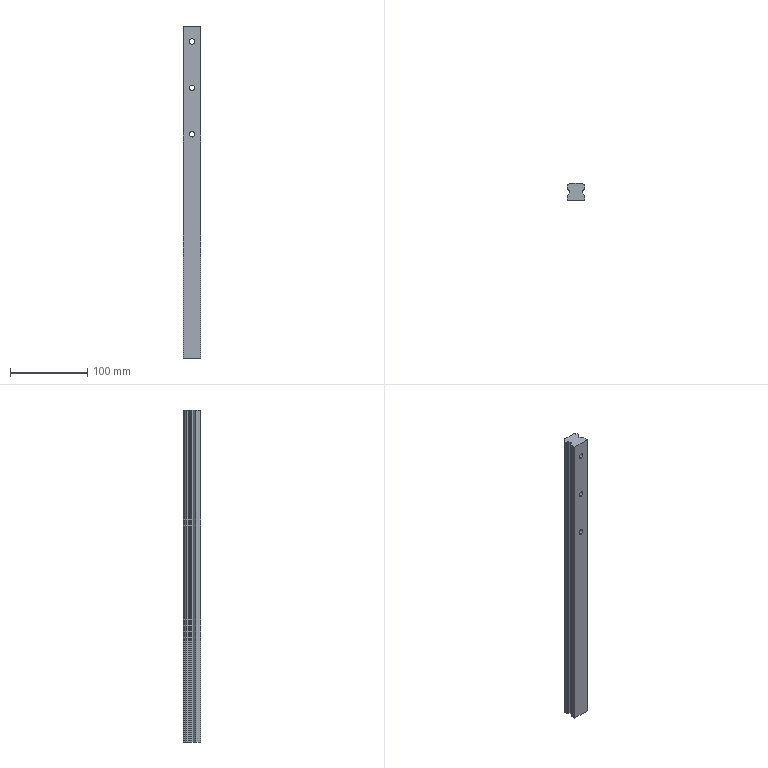Part | STEP file | 1 solid | 41 faces | box 23 x 22 x 429 mm | volume 189571 mm3 | plane 23 | cylinder 18 | commonest cylinder face diameters 2.258 x6 7 x6 11 x6
STEP:
#1=CARTESIAN_POINT('',(0.,-5.6,56.5));
#2=VERTEX_POINT('',#1);
#3=CARTESIAN_POINT('',(0.,-5.6,63.5));
#4=VERTEX_POINT('',#3);
#5=CARTESIAN_POINT('',(0.,-5.6,60.));
#6=DIRECTION('',(0.,1.,0.));
#7=DIRECTION('',(0.,0.,1.));
#8=AXIS2_PLACEMENT_3D('',#5,#6,#7);
#9=CIRCLE('',#8,3.5);
#10=EDGE_CURVE('',#2,#4,#9,.T.);
#11=ORIENTED_EDGE('',*,*,#10,.F.);
#12=CARTESIAN_POINT('',(0.,7.4,56.5));
#13=VERTEX_POINT('',#12);
#14=CARTESIAN_POINT('',(0.,16.4,56.5));
#15=DIRECTION('',(0.,1.,0.));
#16=VECTOR('',#15,1000.);
#17=LINE('',#14,#16);
#18=EDGE_CURVE('',#2,#13,#17,.T.);
#19=ORIENTED_EDGE('',*,*,#18,.T.);
#20=CARTESIAN_POINT('',(0.,7.4,63.5));
#21=VERTEX_POINT('',#20);
#22=CARTESIAN_POINT('',(0.,7.4,60.));
#23=DIRECTION('',(0.,-1.,0.));
#24=DIRECTION('',(0.,0.,1.));
#25=AXIS2_PLACEMENT_3D('',#22,#23,#24);
#26=CIRCLE('',#25,3.5);
#27=EDGE_CURVE('',#21,#13,#26,.T.);
#28=ORIENTED_EDGE('',*,*,#27,.F.);
#29=CARTESIAN_POINT('',(0.,16.4,63.5));
#30=DIRECTION('',(0.,1.,0.));
#31=VECTOR('',#30,1000.);
#32=LINE('',#29,#31);
#33=EDGE_CURVE('',#4,#21,#32,.T.);
#34=ORIENTED_EDGE('',*,*,#33,.F.);
#35=EDGE_LOOP('',(#11,#19,#28,#34));
#36=FACE_OUTER_BOUND('',#35,.T.);
#37=CARTESIAN_POINT('',(0.,16.4,60.));
#38=DIRECTION('',(0.,1.,0.));
#39=DIRECTION('',(0.,0.,1.));
#40=AXIS2_PLACEMENT_3D('',#37,#38,#39);
#41=CYLINDRICAL_SURFACE('',#40,3.5);
#42=ADVANCED_FACE('',(#36),#41,.F.);
#43=CARTESIAN_POINT('',(0.,-5.6,-3.5));
#44=VERTEX_POINT('',#43);
#45=CARTESIAN_POINT('',(0.,-5.6,3.5));
#46=VERTEX_POINT('',#45);
#47=CARTESIAN_POINT('',(0.,-5.6,0.));
#48=DIRECTION('',(0.,1.,0.));
#49=DIRECTION('',(0.,0.,1.));
#50=AXIS2_PLACEMENT_3D('',#47,#48,#49);
#51=CIRCLE('',#50,3.5);
#52=EDGE_CURVE('',#44,#46,#51,.T.);
#53=ORIENTED_EDGE('',*,*,#52,.F.);
#54=CARTESIAN_POINT('',(0.,7.4,-3.5));
#55=VERTEX_POINT('',#54);
#56=CARTESIAN_POINT('',(0.,16.4,-3.5));
#57=DIRECTION('',(0.,1.,0.));
#58=VECTOR('',#57,1000.);
#59=LINE('',#56,#58);
#60=EDGE_CURVE('',#44,#55,#59,.T.);
#61=ORIENTED_EDGE('',*,*,#60,.T.);
#62=CARTESIAN_POINT('',(0.,7.4,3.5));
#63=VERTEX_POINT('',#62);
#64=CARTESIAN_POINT('',(0.,7.4,0.));
#65=DIRECTION('',(0.,-1.,0.));
#66=DIRECTION('',(0.,0.,1.));
#67=AXIS2_PLACEMENT_3D('',#64,#65,#66);
#68=CIRCLE('',#67,3.5);
#69=EDGE_CURVE('',#63,#55,#68,.T.);
#70=ORIENTED_EDGE('',*,*,#69,.F.);
#71=CARTESIAN_POINT('',(0.,16.4,3.5));
#72=DIRECTION('',(0.,1.,0.));
#73=VECTOR('',#72,1000.);
#74=LINE('',#71,#73);
#75=EDGE_CURVE('',#46,#63,#74,.T.);
#76=ORIENTED_EDGE('',*,*,#75,.F.);
#77=EDGE_LOOP('',(#53,#61,#70,#76));
#78=FACE_OUTER_BOUND('',#77,.T.);
#79=CARTESIAN_POINT('',(0.,16.4,0.));
#80=DIRECTION('',(0.,1.,0.));
#81=DIRECTION('',(0.,0.,1.));
#82=AXIS2_PLACEMENT_3D('',#79,#80,#81);
#83=CYLINDRICAL_SURFACE('',#82,3.5);
#84=ADVANCED_FACE('',(#78),#83,.F.);
#85=CARTESIAN_POINT('',(0.,-5.6,-63.5));
#86=VERTEX_POINT('',#85);
#87=CARTESIAN_POINT('',(0.,-5.6,-56.5));
#88=VERTEX_POINT('',#87);
#89=CARTESIAN_POINT('',(0.,-5.6,-60.));
#90=DIRECTION('',(0.,1.,0.));
#91=DIRECTION('',(0.,0.,1.));
#92=AXIS2_PLACEMENT_3D('',#89,#90,#91);
#93=CIRCLE('',#92,3.5);
#94=EDGE_CURVE('',#86,#88,#93,.T.);
#95=ORIENTED_EDGE('',*,*,#94,.F.);
#96=CARTESIAN_POINT('',(0.,7.4,-63.5));
#97=VERTEX_POINT('',#96);
#98=CARTESIAN_POINT('',(0.,16.4,-63.5));
#99=DIRECTION('',(0.,1.,0.));
#100=VECTOR('',#99,1000.);
#101=LINE('',#98,#100);
#102=EDGE_CURVE('',#86,#97,#101,.T.);
#103=ORIENTED_EDGE('',*,*,#102,.T.);
#104=CARTESIAN_POINT('',(0.,7.4,-56.5));
#105=VERTEX_POINT('',#104);
#106=CARTESIAN_POINT('',(0.,7.4,-60.));
#107=DIRECTION('',(0.,-1.,0.));
#108=DIRECTION('',(0.,0.,1.));
#109=AXIS2_PLACEMENT_3D('',#106,#107,#108);
#110=CIRCLE('',#109,3.5);
#111=EDGE_CURVE('',#105,#97,#110,.T.);
#112=ORIENTED_EDGE('',*,*,#111,.F.);
#113=CARTESIAN_POINT('',(0.,16.4,-56.5));
#114=DIRECTION('',(0.,1.,0.));
#115=VECTOR('',#114,1000.);
#116=LINE('',#113,#115);
#117=EDGE_CURVE('',#88,#105,#116,.T.);
#118=ORIENTED_EDGE('',*,*,#117,.F.);
#119=EDGE_LOOP('',(#95,#103,#112,#118));
#120=FACE_OUTER_BOUND('',#119,.T.);
#121=CARTESIAN_POINT('',(0.,16.4,-60.));
#122=DIRECTION('',(0.,1.,0.));
#123=DIRECTION('',(0.,0.,1.));
#124=AXIS2_PLACEMENT_3D('',#121,#122,#123);
#125=CYLINDRICAL_SURFACE('',#124,3.5);
#126=ADVANCED_FACE('',(#120),#125,.F.);
#127=CARTESIAN_POINT('',(-9.204,7.727,-349.));
#128=VERTEX_POINT('',#127);
#129=CARTESIAN_POINT('',(-10.352,8.856,-349.));
#130=VERTEX_POINT('',#129);
#131=CARTESIAN_POINT('',(-10.333,7.727,-349.));
#132=DIRECTION('',(0.,0.,1.));
#133=DIRECTION('',(-1.,0.,0.));
#134=AXIS2_PLACEMENT_3D('',#131,#132,#133);
#135=CIRCLE('',#134,1.129);
#136=EDGE_CURVE('',#128,#130,#135,.T.);
#137=ORIENTED_EDGE('',*,*,#136,.F.);
#138=CARTESIAN_POINT('',(-9.204,7.727,80.));
#139=VERTEX_POINT('',#138);
#140=CARTESIAN_POINT('',(-9.204,7.727,-80.));
#141=DIRECTION('',(0.,0.,1.));
#142=VECTOR('',#141,1000.);
#143=LINE('',#140,#142);
#144=EDGE_CURVE('',#128,#139,#143,.T.);
#145=ORIENTED_EDGE('',*,*,#144,.T.);
#146=CARTESIAN_POINT('',(-10.352,8.856,80.));
#147=VERTEX_POINT('',#146);
#148=CARTESIAN_POINT('',(-10.333,7.727,80.));
#149=DIRECTION('',(0.,0.,-1.));
#150=DIRECTION('',(1.,0.,0.));
#151=AXIS2_PLACEMENT_3D('',#148,#149,#150);
#152=CIRCLE('',#151,1.129);
#153=EDGE_CURVE('',#147,#139,#152,.T.);
#154=ORIENTED_EDGE('',*,*,#153,.F.);
#155=CARTESIAN_POINT('',(-10.352,8.856,-80.));
#156=DIRECTION('',(0.,0.,1.));
#157=VECTOR('',#156,1000.);
#158=LINE('',#155,#157);
#159=EDGE_CURVE('',#130,#147,#158,.T.);
#160=ORIENTED_EDGE('',*,*,#159,.F.);
#161=EDGE_LOOP('',(#137,#145,#154,#160));
#162=FACE_OUTER_BOUND('',#161,.T.);
#163=CARTESIAN_POINT('',(-10.333,7.727,-80.));
#164=DIRECTION('',(0.,0.,1.));
#165=DIRECTION('',(1.,0.,0.));
#166=AXIS2_PLACEMENT_3D('',#163,#164,#165);
#167=CYLINDRICAL_SURFACE('',#166,1.129);
#168=ADVANCED_FACE('',(#162),#167,.F.);
#169=CARTESIAN_POINT('',(-9.204,15.233,-349.));
#170=VERTEX_POINT('',#169);
#171=CARTESIAN_POINT('',(-9.204,15.252,-349.));
#172=VERTEX_POINT('',#171);
#173=CARTESIAN_POINT('',(-10.333,15.233,-349.));
#174=DIRECTION('',(0.,0.,1.));
#175=DIRECTION('',(-1.,0.,0.));
#176=AXIS2_PLACEMENT_3D('',#173,#174,#175);
#177=CIRCLE('',#176,1.129);
#178=EDGE_CURVE('',#170,#172,#177,.T.);
#179=ORIENTED_EDGE('',*,*,#178,.F.);
#180=CARTESIAN_POINT('',(-9.204,15.233,80.));
#181=VERTEX_POINT('',#180);
#182=CARTESIAN_POINT('',(-9.204,15.233,-80.));
#183=DIRECTION('',(0.,0.,1.));
#184=VECTOR('',#183,1000.);
#185=LINE('',#182,#184);
#186=EDGE_CURVE('',#170,#181,#185,.T.);
#187=ORIENTED_EDGE('',*,*,#186,.T.);
#188=CARTESIAN_POINT('',(-9.204,15.252,80.));
#189=VERTEX_POINT('',#188);
#190=CARTESIAN_POINT('',(-10.333,15.233,80.));
#191=DIRECTION('',(0.,0.,-1.));
#192=DIRECTION('',(1.,0.,0.));
#193=AXIS2_PLACEMENT_3D('',#190,#191,#192);
#194=CIRCLE('',#193,1.129);
#195=EDGE_CURVE('',#189,#181,#194,.T.);
#196=ORIENTED_EDGE('',*,*,#195,.F.);
#197=CARTESIAN_POINT('',(-9.204,15.252,-80.));
#198=DIRECTION('',(0.,0.,1.));
#199=VECTOR('',#198,1000.);
#200=LINE('',#197,#199);
#201=EDGE_CURVE('',#172,#189,#200,.T.);
#202=ORIENTED_EDGE('',*,*,#201,.F.);
#203=EDGE_LOOP('',(#179,#187,#196,#202));
#204=FACE_OUTER_BOUND('',#203,.T.);
#205=CARTESIAN_POINT('',(-10.333,15.233,-80.));
#206=DIRECTION('',(0.,0.,1.));
#207=DIRECTION('',(1.,0.,0.));
#208=AXIS2_PLACEMENT_3D('',#205,#206,#207);
#209=CYLINDRICAL_SURFACE('',#208,1.129);
#210=ADVANCED_FACE('',(#204),#209,.F.);
#211=CARTESIAN_POINT('',(0.,7.4,65.5));
#212=VERTEX_POINT('',#211);
#213=CARTESIAN_POINT('',(0.,7.4,54.5));
#214=VERTEX_POINT('',#213);
#215=CARTESIAN_POINT('',(0.,7.4,60.));
#216=DIRECTION('',(0.,-1.,0.));
#217=DIRECTION('',(0.,0.,1.));
#218=AXIS2_PLACEMENT_3D('',#215,#216,#217);
#219=CIRCLE('',#218,5.5);
#220=EDGE_CURVE('',#212,#214,#219,.T.);
#221=ORIENTED_EDGE('',*,*,#220,.T.);
#222=CARTESIAN_POINT('',(0.,16.4,54.5));
#223=VERTEX_POINT('',#222);
#224=CARTESIAN_POINT('',(0.,16.4,54.5));
#225=DIRECTION('',(0.,1.,0.));
#226=VECTOR('',#225,1000.);
#227=LINE('',#224,#226);
#228=EDGE_CURVE('',#214,#223,#227,.T.);
#229=ORIENTED_EDGE('',*,*,#228,.T.);
#230=CARTESIAN_POINT('',(0.,16.4,65.5));
#231=VERTEX_POINT('',#230);
#232=CARTESIAN_POINT('',(0.,16.4,60.));
#233=DIRECTION('',(0.,-1.,0.));
#234=DIRECTION('',(0.,0.,1.));
#235=AXIS2_PLACEMENT_3D('',#232,#233,#234);
#236=CIRCLE('',#235,5.5);
#237=EDGE_CURVE('',#231,#223,#236,.T.);
#238=ORIENTED_EDGE('',*,*,#237,.F.);
#239=CARTESIAN_POINT('',(0.,16.4,65.5));
#240=DIRECTION('',(0.,1.,0.));
#241=VECTOR('',#240,1000.);
#242=LINE('',#239,#241);
#243=EDGE_CURVE('',#212,#231,#242,.T.);
#244=ORIENTED_EDGE('',*,*,#243,.F.);
#245=EDGE_LOOP('',(#221,#229,#238,#244));
#246=FACE_OUTER_BOUND('',#245,.T.);
#247=CARTESIAN_POINT('',(0.,16.4,60.));
#248=DIRECTION('',(0.,1.,0.));
#249=DIRECTION('',(0.,0.,1.));
#250=AXIS2_PLACEMENT_3D('',#247,#248,#249);
#251=CYLINDRICAL_SURFACE('',#250,5.5);
#252=ADVANCED_FACE('',(#246),#251,.F.);
#253=CARTESIAN_POINT('',(0.,7.4,5.5));
#254=VERTEX_POINT('',#253);
#255=CARTESIAN_POINT('',(0.,7.4,-5.5));
#256=VERTEX_POINT('',#255);
#257=CARTESIAN_POINT('',(0.,7.4,0.));
#258=DIRECTION('',(0.,-1.,0.));
#259=DIRECTION('',(0.,0.,1.));
#260=AXIS2_PLACEMENT_3D('',#257,#258,#259);
#261=CIRCLE('',#260,5.5);
#262=EDGE_CURVE('',#254,#256,#261,.T.);
#263=ORIENTED_EDGE('',*,*,#262,.T.);
#264=CARTESIAN_POINT('',(0.,16.4,-5.5));
#265=VERTEX_POINT('',#264);
#266=CARTESIAN_POINT('',(0.,16.4,-5.5));
#267=DIRECTION('',(0.,1.,0.));
#268=VECTOR('',#267,1000.);
#269=LINE('',#266,#268);
#270=EDGE_CURVE('',#256,#265,#269,.T.);
#271=ORIENTED_EDGE('',*,*,#270,.T.);
#272=CARTESIAN_POINT('',(0.,16.4,5.5));
#273=VERTEX_POINT('',#272);
#274=CARTESIAN_POINT('',(0.,16.4,0.));
#275=DIRECTION('',(0.,-1.,0.));
#276=DIRECTION('',(0.,0.,1.));
#277=AXIS2_PLACEMENT_3D('',#274,#275,#276);
#278=CIRCLE('',#277,5.5);
#279=EDGE_CURVE('',#273,#265,#278,.T.);
#280=ORIENTED_EDGE('',*,*,#279,.F.);
#281=CARTESIAN_POINT('',(0.,16.4,5.5));
#282=DIRECTION('',(0.,1.,0.));
#283=VECTOR('',#282,1000.);
#284=LINE('',#281,#283);
#285=EDGE_CURVE('',#254,#273,#284,.T.);
#286=ORIENTED_EDGE('',*,*,#285,.F.);
#287=EDGE_LOOP('',(#263,#271,#280,#286));
#288=FACE_OUTER_BOUND('',#287,.T.);
#289=CARTESIAN_POINT('',(0.,16.4,0.));
#290=DIRECTION('',(0.,1.,0.));
#291=DIRECTION('',(0.,0.,1.));
#292=AXIS2_PLACEMENT_3D('',#289,#290,#291);
#293=CYLINDRICAL_SURFACE('',#292,5.5);
#294=ADVANCED_FACE('',(#288),#293,.F.);
#295=CARTESIAN_POINT('',(0.,7.4,-54.5));
#296=VERTEX_POINT('',#295);
#297=CARTESIAN_POINT('',(0.,7.4,-65.5));
#298=VERTEX_POINT('',#297);
#299=CARTESIAN_POINT('',(0.,7.4,-60.));
#300=DIRECTION('',(0.,-1.,0.));
#301=DIRECTION('',(0.,0.,1.));
#302=AXIS2_PLACEMENT_3D('',#299,#300,#301);
#303=CIRCLE('',#302,5.5);
#304=EDGE_CURVE('',#296,#298,#303,.T.);
#305=ORIENTED_EDGE('',*,*,#304,.T.);
#306=CARTESIAN_POINT('',(0.,16.4,-65.5));
#307=VERTEX_POINT('',#306);
#308=CARTESIAN_POINT('',(0.,16.4,-65.5));
#309=DIRECTION('',(0.,1.,0.));
#310=VECTOR('',#309,1000.);
#311=LINE('',#308,#310);
#312=EDGE_CURVE('',#298,#307,#311,.T.);
#313=ORIENTED_EDGE('',*,*,#312,.T.);
#314=CARTESIAN_POINT('',(0.,16.4,-54.5));
#315=VERTEX_POINT('',#314);
#316=CARTESIAN_POINT('',(0.,16.4,-60.));
#317=DIRECTION('',(0.,-1.,0.));
#318=DIRECTION('',(0.,0.,1.));
#319=AXIS2_PLACEMENT_3D('',#316,#317,#318);
#320=CIRCLE('',#319,5.5);
#321=EDGE_CURVE('',#315,#307,#320,.T.);
#322=ORIENTED_EDGE('',*,*,#321,.F.);
#323=CARTESIAN_POINT('',(0.,16.4,-54.5));
#324=DIRECTION('',(0.,1.,0.));
#325=VECTOR('',#324,1000.);
#326=LINE('',#323,#325);
#327=EDGE_CURVE('',#296,#315,#326,.T.);
#328=ORIENTED_EDGE('',*,*,#327,.F.);
#329=EDGE_LOOP('',(#305,#313,#322,#328));
#330=FACE_OUTER_BOUND('',#329,.T.);
#331=CARTESIAN_POINT('',(0.,16.4,-60.));
#332=DIRECTION('',(0.,1.,0.));
#333=DIRECTION('',(0.,0.,1.));
#334=AXIS2_PLACEMENT_3D('',#331,#332,#333);
#335=CYLINDRICAL_SURFACE('',#334,5.5);
#336=ADVANCED_FACE('',(#330),#335,.F.);
#337=CARTESIAN_POINT('',(-11.5,-5.6,80.));
#338=VERTEX_POINT('',#337);
#339=CARTESIAN_POINT('',(-11.5,-5.6,-349.));
#340=VERTEX_POINT('',#339);
#341=CARTESIAN_POINT('',(-11.5,-5.6,-80.));
#342=DIRECTION('',(0.,0.,-1.));
#343=VECTOR('',#342,1000.);
#344=LINE('',#341,#343);
#345=EDGE_CURVE('',#338,#340,#344,.T.);
#346=ORIENTED_EDGE('',*,*,#345,.T.);
#347=CARTESIAN_POINT('',(11.5,-5.6,-349.));
#348=VERTEX_POINT('',#347);
#349=CARTESIAN_POINT('',(11.5,-5.6,-349.));
#350=DIRECTION('',(-1.,0.,0.));
#351=VECTOR('',#350,1000.);
#352=LINE('',#349,#351);
#353=EDGE_CURVE('',#348,#340,#352,.T.);
#354=ORIENTED_EDGE('',*,*,#353,.F.);
#355=CARTESIAN_POINT('',(11.5,-5.6,80.));
#356=VERTEX_POINT('',#355);
#357=CARTESIAN_POINT('',(11.5,-5.6,-80.));
#358=DIRECTION('',(0.,0.,1.));
#359=VECTOR('',#358,1000.);
#360=LINE('',#357,#359);
#361=EDGE_CURVE('',#348,#356,#360,.T.);
#362=ORIENTED_EDGE('',*,*,#361,.T.);
#363=CARTESIAN_POINT('',(-11.5,-5.6,80.));
#364=DIRECTION('',(-1.,0.,0.));
#365=VECTOR('',#364,1000.);
#366=LINE('',#363,#365);
#367=EDGE_CURVE('',#356,#338,#366,.T.);
#368=ORIENTED_EDGE('',*,*,#367,.T.);
#369=EDGE_LOOP('',(#346,#354,#362,#368));
#370=FACE_OUTER_BOUND('',#369,.T.);
#371=CARTESIAN_POINT('',(0.,-5.6,60.));
#372=DIRECTION('',(0.,1.,0.));
#373=DIRECTION('',(0.,0.,1.));
#374=AXIS2_PLACEMENT_3D('',#371,#372,#373);
#375=CIRCLE('',#374,3.5);
#376=EDGE_CURVE('',#4,#2,#375,.T.);
#377=ORIENTED_EDGE('',*,*,#376,.T.);
#378=ORIENTED_EDGE('',*,*,#10,.T.);
#379=EDGE_LOOP('',(#377,#378));
#380=FACE_BOUND('',#379,.T.);
#381=CARTESIAN_POINT('',(0.,-5.6,0.));
#382=DIRECTION('',(0.,1.,0.));
#383=DIRECTION('',(0.,0.,1.));
#384=AXIS2_PLACEMENT_3D('',#381,#382,#383);
#385=CIRCLE('',#384,3.5);
#386=EDGE_CURVE('',#46,#44,#385,.T.);
#387=ORIENTED_EDGE('',*,*,#386,.T.);
#388=ORIENTED_EDGE('',*,*,#52,.T.);
#389=EDGE_LOOP('',(#387,#388));
#390=FACE_BOUND('',#389,.T.);
#391=CARTESIAN_POINT('',(0.,-5.6,-60.));
#392=DIRECTION('',(0.,1.,0.));
#393=DIRECTION('',(0.,0.,1.));
#394=AXIS2_PLACEMENT_3D('',#391,#392,#393);
#395=CIRCLE('',#394,3.5);
#396=EDGE_CURVE('',#88,#86,#395,.T.);
#397=ORIENTED_EDGE('',*,*,#396,.T.);
#398=ORIENTED_EDGE('',*,*,#94,.T.);
#399=EDGE_LOOP('',(#397,#398));
#400=FACE_BOUND('',#399,.T.);
#401=CARTESIAN_POINT('',(-11.5,-5.6,-80.));
#402=DIRECTION('',(0.,-1.,0.));
#403=DIRECTION('',(0.,0.,-1.));
#404=AXIS2_PLACEMENT_3D('',#401,#402,#403);
#405=PLANE('',#404);
#406=ADVANCED_FACE('',(#370,#380,#390,#400),#405,.T.);
#407=CARTESIAN_POINT('',(-11.5,0.575,80.));
#408=VERTEX_POINT('',#407);
#409=CARTESIAN_POINT('',(-11.5,0.575,-349.));
#410=VERTEX_POINT('',#409);
#411=CARTESIAN_POINT('',(-11.5,0.575,-80.));
#412=DIRECTION('',(0.,0.,-1.));
#413=VECTOR('',#412,1000.);
#414=LINE('',#411,#413);
#415=EDGE_CURVE('',#408,#410,#414,.T.);
#416=ORIENTED_EDGE('',*,*,#415,.T.);
#417=CARTESIAN_POINT('',(-11.5,-5.6,-349.));
#418=DIRECTION('',(0.,1.,0.));
#419=VECTOR('',#418,1000.);
#420=LINE('',#417,#419);
#421=EDGE_CURVE('',#340,#410,#420,.T.);
#422=ORIENTED_EDGE('',*,*,#421,.F.);
#423=ORIENTED_EDGE('',*,*,#345,.F.);
#424=CARTESIAN_POINT('',(-11.5,-5.6,80.));
#425=DIRECTION('',(0.,1.,0.));
#426=VECTOR('',#425,1000.);
#427=LINE('',#424,#426);
#428=EDGE_CURVE('',#338,#408,#427,.T.);
#429=ORIENTED_EDGE('',*,*,#428,.T.);
#430=EDGE_LOOP('',(#416,#422,#423,#429));
#431=FACE_OUTER_BOUND('',#430,.T.);
#432=CARTESIAN_POINT('',(-11.5,-5.6,-80.));
#433=DIRECTION('',(-1.,0.,0.));
#434=DIRECTION('',(0.,-1.,0.));
#435=AXIS2_PLACEMENT_3D('',#432,#433,#434);
#436=PLANE('',#435);
#437=ADVANCED_FACE('',(#431),#436,.T.);
#438=CARTESIAN_POINT('',(10.352,14.104,80.));
#439=VERTEX_POINT('',#438);
#440=CARTESIAN_POINT('',(11.5,12.956,80.));
#441=VERTEX_POINT('',#440);
#442=CARTESIAN_POINT('',(11.5,12.956,80.));
#443=DIRECTION('',(0.7071,-0.7071,0.));
#444=VECTOR('',#443,1000.);
#445=LINE('',#442,#444);
#446=EDGE_CURVE('',#439,#441,#445,.T.);
#447=ORIENTED_EDGE('',*,*,#446,.F.);
#448=CARTESIAN_POINT('',(9.204,15.252,80.));
#449=VERTEX_POINT('',#448);
#450=CARTESIAN_POINT('',(10.333,15.233,80.));
#451=DIRECTION('',(0.,0.,-1.));
#452=DIRECTION('',(1.,0.,0.));
#453=AXIS2_PLACEMENT_3D('',#450,#451,#452);
#454=CIRCLE('',#453,1.129);
#455=EDGE_CURVE('',#439,#449,#454,.T.);
#456=ORIENTED_EDGE('',*,*,#455,.T.);
#457=CARTESIAN_POINT('',(8.056,16.4,80.));
#458=VERTEX_POINT('',#457);
#459=CARTESIAN_POINT('',(9.204,15.252,80.));
#460=DIRECTION('',(0.7071,-0.7071,0.));
#461=VECTOR('',#460,1000.);
#462=LINE('',#459,#461);
#463=EDGE_CURVE('',#458,#449,#462,.T.);
#464=ORIENTED_EDGE('',*,*,#463,.F.);
#465=CARTESIAN_POINT('',(-8.056,16.4,80.));
#466=VERTEX_POINT('',#465);
#467=CARTESIAN_POINT('',(-10.333,16.4,80.));
#468=DIRECTION('',(-1.,0.,0.));
#469=VECTOR('',#468,1000.);
#470=LINE('',#467,#469);
#471=EDGE_CURVE('',#458,#466,#470,.T.);
#472=ORIENTED_EDGE('',*,*,#471,.T.);
#473=CARTESIAN_POINT('',(-9.204,15.252,80.));
#474=DIRECTION('',(0.7071,0.7071,0.));
#475=VECTOR('',#474,1000.);
#476=LINE('',#473,#475);
#477=EDGE_CURVE('',#189,#466,#476,.T.);
#478=ORIENTED_EDGE('',*,*,#477,.F.);
#479=ORIENTED_EDGE('',*,*,#195,.T.);
#480=CARTESIAN_POINT('',(-10.352,14.104,80.));
#481=VERTEX_POINT('',#480);
#482=CARTESIAN_POINT('',(-10.333,15.233,80.));
#483=DIRECTION('',(0.,0.,-1.));
#484=DIRECTION('',(1.,0.,0.));
#485=AXIS2_PLACEMENT_3D('',#482,#483,#484);
#486=CIRCLE('',#485,1.129);
#487=EDGE_CURVE('',#181,#481,#486,.T.);
#488=ORIENTED_EDGE('',*,*,#487,.T.);
#489=CARTESIAN_POINT('',(-11.5,12.956,80.));
#490=VERTEX_POINT('',#489);
#491=CARTESIAN_POINT('',(-11.5,12.956,80.));
#492=DIRECTION('',(0.7071,0.7071,0.));
#493=VECTOR('',#492,1000.);
#494=LINE('',#491,#493);
#495=EDGE_CURVE('',#490,#481,#494,.T.);
#496=ORIENTED_EDGE('',*,*,#495,.F.);
#497=CARTESIAN_POINT('',(-11.5,10.004,80.));
#498=VERTEX_POINT('',#497);
#499=CARTESIAN_POINT('',(-11.5,15.233,80.));
#500=DIRECTION('',(0.,-1.,0.));
#501=VECTOR('',#500,1000.);
#502=LINE('',#499,#501);
#503=EDGE_CURVE('',#490,#498,#502,.T.);
#504=ORIENTED_EDGE('',*,*,#503,.T.);
#505=CARTESIAN_POINT('',(-10.352,8.856,80.));
#506=DIRECTION('',(-0.7071,0.7071,0.));
#507=VECTOR('',#506,1000.);
#508=LINE('',#505,#507);
#509=EDGE_CURVE('',#147,#498,#508,.T.);
#510=ORIENTED_EDGE('',*,*,#509,.F.);
#511=ORIENTED_EDGE('',*,*,#153,.T.);
#512=CARTESIAN_POINT('',(-9.204,7.708,80.));
#513=VERTEX_POINT('',#512);
#514=CARTESIAN_POINT('',(-10.333,7.727,80.));
#515=DIRECTION('',(0.,0.,-1.));
#516=DIRECTION('',(1.,0.,0.));
#517=AXIS2_PLACEMENT_3D('',#514,#515,#516);
#518=CIRCLE('',#517,1.129);
#519=EDGE_CURVE('',#139,#513,#518,.T.);
#520=ORIENTED_EDGE('',*,*,#519,.T.);
#521=CARTESIAN_POINT('',(-8.056,6.56,80.));
#522=VERTEX_POINT('',#521);
#523=CARTESIAN_POINT('',(-8.056,6.56,80.));
#524=DIRECTION('',(-0.7071,0.7071,0.));
#525=VECTOR('',#524,1000.);
#526=LINE('',#523,#525);
#527=EDGE_CURVE('',#522,#513,#526,.T.);
#528=ORIENTED_EDGE('',*,*,#527,.F.);
#529=CARTESIAN_POINT('',(-8.056,4.019,80.));
#530=VERTEX_POINT('',#529);
#531=CARTESIAN_POINT('',(-8.056,15.233,80.));
#532=DIRECTION('',(0.,-1.,0.));
#533=VECTOR('',#532,1000.);
#534=LINE('',#531,#533);
#535=EDGE_CURVE('',#522,#530,#534,.T.);
#536=ORIENTED_EDGE('',*,*,#535,.T.);
#537=CARTESIAN_POINT('',(-8.056,4.019,80.));
#538=DIRECTION('',(-0.7071,-0.7071,0.));
#539=VECTOR('',#538,1000.);
#540=LINE('',#537,#539);
#541=EDGE_CURVE('',#530,#408,#540,.T.);
#542=ORIENTED_EDGE('',*,*,#541,.T.);
#543=ORIENTED_EDGE('',*,*,#428,.F.);
#544=ORIENTED_EDGE('',*,*,#367,.F.);
#545=CARTESIAN_POINT('',(11.5,0.575,80.));
#546=VERTEX_POINT('',#545);
#547=CARTESIAN_POINT('',(11.5,15.233,80.));
#548=DIRECTION('',(0.,1.,0.));
#549=VECTOR('',#548,1000.);
#550=LINE('',#547,#549);
#551=EDGE_CURVE('',#356,#546,#550,.T.);
#552=ORIENTED_EDGE('',*,*,#551,.T.);
#553=CARTESIAN_POINT('',(8.056,4.019,80.));
#554=VERTEX_POINT('',#553);
#555=CARTESIAN_POINT('',(11.5,0.575,80.));
#556=DIRECTION('',(-0.7071,0.7071,0.));
#557=VECTOR('',#556,1000.);
#558=LINE('',#555,#557);
#559=EDGE_CURVE('',#546,#554,#558,.T.);
#560=ORIENTED_EDGE('',*,*,#559,.T.);
#561=CARTESIAN_POINT('',(8.056,6.56,80.));
#562=VERTEX_POINT('',#561);
#563=CARTESIAN_POINT('',(8.056,15.233,80.));
#564=DIRECTION('',(0.,1.,0.));
#565=VECTOR('',#564,1000.);
#566=LINE('',#563,#565);
#567=EDGE_CURVE('',#554,#562,#566,.T.);
#568=ORIENTED_EDGE('',*,*,#567,.T.);
#569=CARTESIAN_POINT('',(9.204,7.708,80.));
#570=VERTEX_POINT('',#569);
#571=CARTESIAN_POINT('',(8.056,6.56,80.));
#572=DIRECTION('',(-0.7071,-0.7071,0.));
#573=VECTOR('',#572,1000.);
#574=LINE('',#571,#573);
#575=EDGE_CURVE('',#570,#562,#574,.T.);
#576=ORIENTED_EDGE('',*,*,#575,.F.);
#577=CARTESIAN_POINT('',(10.352,8.856,80.));
#578=VERTEX_POINT('',#577);
#579=CARTESIAN_POINT('',(10.333,7.727,80.));
#580=DIRECTION('',(0.,0.,-1.));
#581=DIRECTION('',(1.,0.,0.));
#582=AXIS2_PLACEMENT_3D('',#579,#580,#581);
#583=CIRCLE('',#582,1.129);
#584=EDGE_CURVE('',#570,#578,#583,.T.);
#585=ORIENTED_EDGE('',*,*,#584,.T.);
#586=CARTESIAN_POINT('',(11.5,10.004,80.));
#587=VERTEX_POINT('',#586);
#588=CARTESIAN_POINT('',(10.352,8.856,80.));
#589=DIRECTION('',(-0.7071,-0.7071,0.));
#590=VECTOR('',#589,1000.);
#591=LINE('',#588,#590);
#592=EDGE_CURVE('',#587,#578,#591,.T.);
#593=ORIENTED_EDGE('',*,*,#592,.F.);
#594=CARTESIAN_POINT('',(11.5,15.233,80.));
#595=DIRECTION('',(0.,1.,0.));
#596=VECTOR('',#595,1000.);
#597=LINE('',#594,#596);
#598=EDGE_CURVE('',#587,#441,#597,.T.);
#599=ORIENTED_EDGE('',*,*,#598,.T.);
#600=EDGE_LOOP('',(#447,#456,#464,#472,#478,#479,#488,#496,#504,#510,#511,#520,#528,#536,#542,#543,#544,#552,#560,#568,#576,#585,#593,#599));
#601=FACE_OUTER_BOUND('',#600,.T.);
#602=CARTESIAN_POINT('',(-10.333,15.233,80.));
#603=DIRECTION('',(0.,0.,1.));
#604=DIRECTION('',(1.,0.,0.));
#605=AXIS2_PLACEMENT_3D('',#602,#603,#604);
#606=PLANE('',#605);
#607=ADVANCED_FACE('',(#601),#606,.T.);
#608=ORIENTED_EDGE('',*,*,#361,.F.);
#609=CARTESIAN_POINT('',(11.5,0.575,-349.));
#610=VERTEX_POINT('',#609);
#611=CARTESIAN_POINT('',(11.5,0.575,-349.));
#612=DIRECTION('',(0.,-1.,0.));
#613=VECTOR('',#612,1000.);
#614=LINE('',#611,#613);
#615=EDGE_CURVE('',#610,#348,#614,.T.);
#616=ORIENTED_EDGE('',*,*,#615,.F.);
#617=CARTESIAN_POINT('',(11.5,0.575,-80.));
#618=DIRECTION('',(0.,0.,1.));
#619=VECTOR('',#618,1000.);
#620=LINE('',#617,#619);
#621=EDGE_CURVE('',#610,#546,#620,.T.);
#622=ORIENTED_EDGE('',*,*,#621,.T.);
#623=ORIENTED_EDGE('',*,*,#551,.F.);
#624=EDGE_LOOP('',(#608,#616,#622,#623));
#625=FACE_OUTER_BOUND('',#624,.T.);
#626=CARTESIAN_POINT('',(11.5,-5.6,-80.));
#627=DIRECTION('',(1.,0.,0.));
#628=DIRECTION('',(0.,1.,0.));
#629=AXIS2_PLACEMENT_3D('',#626,#627,#628);
#630=PLANE('',#629);
#631=ADVANCED_FACE('',(#625),#630,.T.);
#632=ORIENTED_EDGE('',*,*,#18,.F.);
#633=ORIENTED_EDGE('',*,*,#376,.F.);
#634=ORIENTED_EDGE('',*,*,#33,.T.);
#635=CARTESIAN_POINT('',(0.,7.4,60.));
#636=DIRECTION('',(0.,-1.,0.));
#637=DIRECTION('',(0.,0.,1.));
#638=AXIS2_PLACEMENT_3D('',#635,#636,#637);
#639=CIRCLE('',#638,3.5);
#640=EDGE_CURVE('',#13,#21,#639,.T.);
#641=ORIENTED_EDGE('',*,*,#640,.F.);
#642=EDGE_LOOP('',(#632,#633,#634,#641));
#643=FACE_OUTER_BOUND('',#642,.T.);
#644=CARTESIAN_POINT('',(0.,16.4,60.));
#645=DIRECTION('',(0.,1.,0.));
#646=DIRECTION('',(0.,0.,1.));
#647=AXIS2_PLACEMENT_3D('',#644,#645,#646);
#648=CYLINDRICAL_SURFACE('',#647,3.5);
#649=ADVANCED_FACE('',(#643),#648,.F.);
#650=ORIENTED_EDGE('',*,*,#60,.F.);
#651=ORIENTED_EDGE('',*,*,#386,.F.);
#652=ORIENTED_EDGE('',*,*,#75,.T.);
#653=CARTESIAN_POINT('',(0.,7.4,0.));
#654=DIRECTION('',(0.,-1.,0.));
#655=DIRECTION('',(0.,0.,1.));
#656=AXIS2_PLACEMENT_3D('',#653,#654,#655);
#657=CIRCLE('',#656,3.5);
#658=EDGE_CURVE('',#55,#63,#657,.T.);
#659=ORIENTED_EDGE('',*,*,#658,.F.);
#660=EDGE_LOOP('',(#650,#651,#652,#659));
#661=FACE_OUTER_BOUND('',#660,.T.);
#662=CARTESIAN_POINT('',(0.,16.4,0.));
#663=DIRECTION('',(0.,1.,0.));
#664=DIRECTION('',(0.,0.,1.));
#665=AXIS2_PLACEMENT_3D('',#662,#663,#664);
#666=CYLINDRICAL_SURFACE('',#665,3.5);
#667=ADVANCED_FACE('',(#661),#666,.F.);
#668=ORIENTED_EDGE('',*,*,#102,.F.);
#669=ORIENTED_EDGE('',*,*,#396,.F.);
#670=ORIENTED_EDGE('',*,*,#117,.T.);
#671=CARTESIAN_POINT('',(0.,7.4,-60.));
#672=DIRECTION('',(0.,-1.,0.));
#673=DIRECTION('',(0.,0.,1.));
#674=AXIS2_PLACEMENT_3D('',#671,#672,#673);
#675=CIRCLE('',#674,3.5);
#676=EDGE_CURVE('',#97,#105,#675,.T.);
#677=ORIENTED_EDGE('',*,*,#676,.F.);
#678=EDGE_LOOP('',(#668,#669,#670,#677));
#679=FACE_OUTER_BOUND('',#678,.T.);
#680=CARTESIAN_POINT('',(0.,16.4,-60.));
#681=DIRECTION('',(0.,1.,0.));
#682=DIRECTION('',(0.,0.,1.));
#683=AXIS2_PLACEMENT_3D('',#680,#681,#682);
#684=CYLINDRICAL_SURFACE('',#683,3.5);
#685=ADVANCED_FACE('',(#679),#684,.F.);
#686=ORIENTED_EDGE('',*,*,#455,.F.);
#687=CARTESIAN_POINT('',(10.352,14.104,-349.));
#688=VERTEX_POINT('',#687);
#689=CARTESIAN_POINT('',(10.352,14.104,-80.));
#690=DIRECTION('',(0.,0.,1.));
#691=VECTOR('',#690,1000.);
#692=LINE('',#689,#691);
#693=EDGE_CURVE('',#688,#439,#692,.T.);
#694=ORIENTED_EDGE('',*,*,#693,.F.);
#695=CARTESIAN_POINT('',(9.204,15.252,-349.));
#696=VERTEX_POINT('',#695);
#697=CARTESIAN_POINT('',(10.333,15.233,-349.));
#698=DIRECTION('',(0.,0.,1.));
#699=DIRECTION('',(-1.,0.,0.));
#700=AXIS2_PLACEMENT_3D('',#697,#698,#699);
#701=CIRCLE('',#700,1.129);
#702=EDGE_CURVE('',#696,#688,#701,.T.);
#703=ORIENTED_EDGE('',*,*,#702,.F.);
#704=CARTESIAN_POINT('',(9.204,15.252,-80.));
#705=DIRECTION('',(0.,0.,-1.));
#706=VECTOR('',#705,1000.);
#707=LINE('',#704,#706);
#708=EDGE_CURVE('',#449,#696,#707,.T.);
#709=ORIENTED_EDGE('',*,*,#708,.F.);
#710=EDGE_LOOP('',(#686,#694,#703,#709));
#711=FACE_OUTER_BOUND('',#710,.T.);
#712=CARTESIAN_POINT('',(10.333,15.233,-80.));
#713=DIRECTION('',(0.,0.,1.));
#714=DIRECTION('',(1.,0.,0.));
#715=AXIS2_PLACEMENT_3D('',#712,#713,#714);
#716=CYLINDRICAL_SURFACE('',#715,1.129);
#717=ADVANCED_FACE('',(#711),#716,.F.);
#718=CARTESIAN_POINT('',(11.5,10.004,-349.));
#719=VERTEX_POINT('',#718);
#720=CARTESIAN_POINT('',(11.5,10.004,-80.));
#721=DIRECTION('',(0.,0.,-1.));
#722=VECTOR('',#721,1000.);
#723=LINE('',#720,#722);
#724=EDGE_CURVE('',#587,#719,#723,.T.);
#725=ORIENTED_EDGE('',*,*,#724,.T.);
#726=CARTESIAN_POINT('',(11.5,12.956,-349.));
#727=VERTEX_POINT('',#726);
#728=CARTESIAN_POINT('',(11.5,12.956,-349.));
#729=DIRECTION('',(0.,-1.,0.));
#730=VECTOR('',#729,1000.);
#731=LINE('',#728,#730);
#732=EDGE_CURVE('',#727,#719,#731,.T.);
#733=ORIENTED_EDGE('',*,*,#732,.F.);
#734=CARTESIAN_POINT('',(11.5,12.956,-80.));
#735=DIRECTION('',(0.,0.,1.));
#736=VECTOR('',#735,1000.);
#737=LINE('',#734,#736);
#738=EDGE_CURVE('',#727,#441,#737,.T.);
#739=ORIENTED_EDGE('',*,*,#738,.T.);
#740=ORIENTED_EDGE('',*,*,#598,.F.);
#741=EDGE_LOOP('',(#725,#733,#739,#740));
#742=FACE_OUTER_BOUND('',#741,.T.);
#743=CARTESIAN_POINT('',(11.5,10.004,-80.));
#744=DIRECTION('',(1.,0.,0.));
#745=DIRECTION('',(0.,0.,-1.));
#746=AXIS2_PLACEMENT_3D('',#743,#744,#745);
#747=PLANE('',#746);
#748=ADVANCED_FACE('',(#742),#747,.T.);
#749=ORIENTED_EDGE('',*,*,#584,.F.);
#750=CARTESIAN_POINT('',(9.204,7.708,-349.));
#751=VERTEX_POINT('',#750);
#752=CARTESIAN_POINT('',(9.204,7.708,-80.));
#753=DIRECTION('',(0.,0.,1.));
#754=VECTOR('',#753,1000.);
#755=LINE('',#752,#754);
#756=EDGE_CURVE('',#751,#570,#755,.T.);
#757=ORIENTED_EDGE('',*,*,#756,.F.);
#758=CARTESIAN_POINT('',(10.352,8.856,-349.));
#759=VERTEX_POINT('',#758);
#760=CARTESIAN_POINT('',(10.333,7.727,-349.));
#761=DIRECTION('',(0.,0.,1.));
#762=DIRECTION('',(-1.,0.,0.));
#763=AXIS2_PLACEMENT_3D('',#760,#761,#762);
#764=CIRCLE('',#763,1.129);
#765=EDGE_CURVE('',#759,#751,#764,.T.);
#766=ORIENTED_EDGE('',*,*,#765,.F.);
#767=CARTESIAN_POINT('',(10.352,8.856,-80.));
#768=DIRECTION('',(0.,0.,-1.));
#769=VECTOR('',#768,1000.);
#770=LINE('',#767,#769);
#771=EDGE_CURVE('',#578,#759,#770,.T.);
#772=ORIENTED_EDGE('',*,*,#771,.F.);
#773=EDGE_LOOP('',(#749,#757,#766,#772));
#774=FACE_OUTER_BOUND('',#773,.T.);
#775=CARTESIAN_POINT('',(10.333,7.727,-80.));
#776=DIRECTION('',(0.,0.,1.));
#777=DIRECTION('',(1.,0.,0.));
#778=AXIS2_PLACEMENT_3D('',#775,#776,#777);
#779=CYLINDRICAL_SURFACE('',#778,1.129);
#780=ADVANCED_FACE('',(#774),#779,.F.);
#781=CARTESIAN_POINT('',(8.056,4.019,-349.));
#782=VERTEX_POINT('',#781);
#783=CARTESIAN_POINT('',(8.056,4.019,-80.));
#784=DIRECTION('',(0.,0.,-1.));
#785=VECTOR('',#784,1000.);
#786=LINE('',#783,#785);
#787=EDGE_CURVE('',#554,#782,#786,.T.);
#788=ORIENTED_EDGE('',*,*,#787,.T.);
#789=CARTESIAN_POINT('',(8.056,6.56,-349.));
#790=VERTEX_POINT('',#789);
#791=CARTESIAN_POINT('',(8.056,6.56,-349.));
#792=DIRECTION('',(0.,-1.,0.));
#793=VECTOR('',#792,1000.);
#794=LINE('',#791,#793);
#795=EDGE_CURVE('',#790,#782,#794,.T.);
#796=ORIENTED_EDGE('',*,*,#795,.F.);
#797=CARTESIAN_POINT('',(8.056,6.56,-80.));
#798=DIRECTION('',(0.,0.,1.));
#799=VECTOR('',#798,1000.);
#800=LINE('',#797,#799);
#801=EDGE_CURVE('',#790,#562,#800,.T.);
#802=ORIENTED_EDGE('',*,*,#801,.T.);
#803=ORIENTED_EDGE('',*,*,#567,.F.);
#804=EDGE_LOOP('',(#788,#796,#802,#803));
#805=FACE_OUTER_BOUND('',#804,.T.);
#806=CARTESIAN_POINT('',(8.056,4.019,-80.));
#807=DIRECTION('',(1.,0.,0.));
#808=DIRECTION('',(0.,0.,-1.));
#809=AXIS2_PLACEMENT_3D('',#806,#807,#808);
#810=PLANE('',#809);
#811=ADVANCED_FACE('',(#805),#810,.T.);
#812=ORIENTED_EDGE('',*,*,#621,.F.);
#813=CARTESIAN_POINT('',(8.056,4.019,-349.));
#814=DIRECTION('',(0.7071,-0.7071,0.));
#815=VECTOR('',#814,1000.);
#816=LINE('',#813,#815);
#817=EDGE_CURVE('',#782,#610,#816,.T.);
#818=ORIENTED_EDGE('',*,*,#817,.F.);
#819=ORIENTED_EDGE('',*,*,#787,.F.);
#820=ORIENTED_EDGE('',*,*,#559,.F.);
#821=EDGE_LOOP('',(#812,#818,#819,#820));
#822=FACE_OUTER_BOUND('',#821,.T.);
#823=CARTESIAN_POINT('',(11.5,0.575,-80.));
#824=DIRECTION('',(0.7071,0.7071,0.));
#825=DIRECTION('',(-0.7071,0.7071,0.));
#826=AXIS2_PLACEMENT_3D('',#823,#824,#825);
#827=PLANE('',#826);
#828=ADVANCED_FACE('',(#822),#827,.T.);
#829=CARTESIAN_POINT('',(-8.056,4.019,-349.));
#830=VERTEX_POINT('',#829);
#831=CARTESIAN_POINT('',(-8.056,4.019,-80.));
#832=DIRECTION('',(0.,0.,-1.));
#833=VECTOR('',#832,1000.);
#834=LINE('',#831,#833);
#835=EDGE_CURVE('',#530,#830,#834,.T.);
#836=ORIENTED_EDGE('',*,*,#835,.T.);
#837=CARTESIAN_POINT('',(-11.5,0.575,-349.));
#838=DIRECTION('',(0.7071,0.7071,0.));
#839=VECTOR('',#838,1000.);
#840=LINE('',#837,#839);
#841=EDGE_CURVE('',#410,#830,#840,.T.);
#842=ORIENTED_EDGE('',*,*,#841,.F.);
#843=ORIENTED_EDGE('',*,*,#415,.F.);
#844=ORIENTED_EDGE('',*,*,#541,.F.);
#845=EDGE_LOOP('',(#836,#842,#843,#844));
#846=FACE_OUTER_BOUND('',#845,.T.);
#847=CARTESIAN_POINT('',(-11.5,0.575,-80.));
#848=DIRECTION('',(-0.7071,0.7071,0.));
#849=DIRECTION('',(-0.7071,-0.7071,0.));
#850=AXIS2_PLACEMENT_3D('',#847,#848,#849);
#851=PLANE('',#850);
#852=ADVANCED_FACE('',(#846),#851,.T.);
#853=CARTESIAN_POINT('',(-8.056,6.56,-349.));
#854=VERTEX_POINT('',#853);
#855=CARTESIAN_POINT('',(-8.056,6.56,-80.));
#856=DIRECTION('',(0.,0.,-1.));
#857=VECTOR('',#856,1000.);
#858=LINE('',#855,#857);
#859=EDGE_CURVE('',#522,#854,#858,.T.);
#860=ORIENTED_EDGE('',*,*,#859,.T.);
#861=CARTESIAN_POINT('',(-8.056,4.019,-349.));
#862=DIRECTION('',(0.,1.,0.));
#863=VECTOR('',#862,1000.);
#864=LINE('',#861,#863);
#865=EDGE_CURVE('',#830,#854,#864,.T.);
#866=ORIENTED_EDGE('',*,*,#865,.F.);
#867=ORIENTED_EDGE('',*,*,#835,.F.);
#868=ORIENTED_EDGE('',*,*,#535,.F.);
#869=EDGE_LOOP('',(#860,#866,#867,#868));
#870=FACE_OUTER_BOUND('',#869,.T.);
#871=CARTESIAN_POINT('',(-8.056,4.019,-80.));
#872=DIRECTION('',(-1.,0.,0.));
#873=DIRECTION('',(0.,-1.,0.));
#874=AXIS2_PLACEMENT_3D('',#871,#872,#873);
#875=PLANE('',#874);
#876=ADVANCED_FACE('',(#870),#875,.T.);
#877=ORIENTED_EDGE('',*,*,#144,.F.);
#878=CARTESIAN_POINT('',(-9.204,7.708,-349.));
#879=VERTEX_POINT('',#878);
#880=CARTESIAN_POINT('',(-10.333,7.727,-349.));
#881=DIRECTION('',(0.,0.,1.));
#882=DIRECTION('',(-1.,0.,0.));
#883=AXIS2_PLACEMENT_3D('',#880,#881,#882);
#884=CIRCLE('',#883,1.129);
#885=EDGE_CURVE('',#879,#128,#884,.T.);
#886=ORIENTED_EDGE('',*,*,#885,.F.);
#887=CARTESIAN_POINT('',(-9.204,7.708,-80.));
#888=DIRECTION('',(0.,0.,-1.));
#889=VECTOR('',#888,1000.);
#890=LINE('',#887,#889);
#891=EDGE_CURVE('',#513,#879,#890,.T.);
#892=ORIENTED_EDGE('',*,*,#891,.F.);
#893=ORIENTED_EDGE('',*,*,#519,.F.);
#894=EDGE_LOOP('',(#877,#886,#892,#893));
#895=FACE_OUTER_BOUND('',#894,.T.);
#896=CARTESIAN_POINT('',(-10.333,7.727,-80.));
#897=DIRECTION('',(0.,0.,1.));
#898=DIRECTION('',(1.,0.,0.));
#899=AXIS2_PLACEMENT_3D('',#896,#897,#898);
#900=CYLINDRICAL_SURFACE('',#899,1.129);
#901=ADVANCED_FACE('',(#895),#900,.F.);
#902=CARTESIAN_POINT('',(-11.5,12.956,-349.));
#903=VERTEX_POINT('',#902);
#904=CARTESIAN_POINT('',(-11.5,12.956,-80.));
#905=DIRECTION('',(0.,0.,-1.));
#906=VECTOR('',#905,1000.);
#907=LINE('',#904,#906);
#908=EDGE_CURVE('',#490,#903,#907,.T.);
#909=ORIENTED_EDGE('',*,*,#908,.T.);
#910=CARTESIAN_POINT('',(-11.5,10.004,-349.));
#911=VERTEX_POINT('',#910);
#912=CARTESIAN_POINT('',(-11.5,10.004,-349.));
#913=DIRECTION('',(0.,1.,0.));
#914=VECTOR('',#913,1000.);
#915=LINE('',#912,#914);
#916=EDGE_CURVE('',#911,#903,#915,.T.);
#917=ORIENTED_EDGE('',*,*,#916,.F.);
#918=CARTESIAN_POINT('',(-11.5,10.004,-80.));
#919=DIRECTION('',(0.,0.,1.));
#920=VECTOR('',#919,1000.);
#921=LINE('',#918,#920);
#922=EDGE_CURVE('',#911,#498,#921,.T.);
#923=ORIENTED_EDGE('',*,*,#922,.T.);
#924=ORIENTED_EDGE('',*,*,#503,.F.);
#925=EDGE_LOOP('',(#909,#917,#923,#924));
#926=FACE_OUTER_BOUND('',#925,.T.);
#927=CARTESIAN_POINT('',(-11.5,10.004,-80.));
#928=DIRECTION('',(-1.,0.,0.));
#929=DIRECTION('',(0.,-1.,0.));
#930=AXIS2_PLACEMENT_3D('',#927,#928,#929);
#931=PLANE('',#930);
#932=ADVANCED_FACE('',(#926),#931,.T.);
#933=ORIENTED_EDGE('',*,*,#186,.F.);
#934=CARTESIAN_POINT('',(-10.352,14.104,-349.));
#935=VERTEX_POINT('',#934);
#936=CARTESIAN_POINT('',(-10.333,15.233,-349.));
#937=DIRECTION('',(0.,0.,1.));
#938=DIRECTION('',(-1.,0.,0.));
#939=AXIS2_PLACEMENT_3D('',#936,#937,#938);
#940=CIRCLE('',#939,1.129);
#941=EDGE_CURVE('',#935,#170,#940,.T.);
#942=ORIENTED_EDGE('',*,*,#941,.F.);
#943=CARTESIAN_POINT('',(-10.352,14.104,-80.));
#944=DIRECTION('',(0.,0.,-1.));
#945=VECTOR('',#944,1000.);
#946=LINE('',#943,#945);
#947=EDGE_CURVE('',#481,#935,#946,.T.);
#948=ORIENTED_EDGE('',*,*,#947,.F.);
#949=ORIENTED_EDGE('',*,*,#487,.F.);
#950=EDGE_LOOP('',(#933,#942,#948,#949));
#951=FACE_OUTER_BOUND('',#950,.T.);
#952=CARTESIAN_POINT('',(-10.333,15.233,-80.));
#953=DIRECTION('',(0.,0.,1.));
#954=DIRECTION('',(1.,0.,0.));
#955=AXIS2_PLACEMENT_3D('',#952,#953,#954);
#956=CYLINDRICAL_SURFACE('',#955,1.129);
#957=ADVANCED_FACE('',(#951),#956,.F.);
#958=CARTESIAN_POINT('',(8.056,16.4,-349.));
#959=VERTEX_POINT('',#958);
#960=CARTESIAN_POINT('',(8.056,16.4,-80.));
#961=DIRECTION('',(0.,0.,-1.));
#962=VECTOR('',#961,1000.);
#963=LINE('',#960,#962);
#964=EDGE_CURVE('',#458,#959,#963,.T.);
#965=ORIENTED_EDGE('',*,*,#964,.T.);
#966=CARTESIAN_POINT('',(-8.056,16.4,-349.));
#967=VERTEX_POINT('',#966);
#968=CARTESIAN_POINT('',(-8.056,16.4,-349.));
#969=DIRECTION('',(1.,0.,0.));
#970=VECTOR('',#969,1000.);
#971=LINE('',#968,#970);
#972=EDGE_CURVE('',#967,#959,#971,.T.);
#973=ORIENTED_EDGE('',*,*,#972,.F.);
#974=CARTESIAN_POINT('',(-8.056,16.4,-80.));
#975=DIRECTION('',(0.,0.,1.));
#976=VECTOR('',#975,1000.);
#977=LINE('',#974,#976);
#978=EDGE_CURVE('',#967,#466,#977,.T.);
#979=ORIENTED_EDGE('',*,*,#978,.T.);
#980=ORIENTED_EDGE('',*,*,#471,.F.);
#981=EDGE_LOOP('',(#965,#973,#979,#980));
#982=FACE_OUTER_BOUND('',#981,.T.);
#983=ORIENTED_EDGE('',*,*,#237,.T.);
#984=CARTESIAN_POINT('',(0.,16.4,60.));
#985=DIRECTION('',(0.,-1.,0.));
#986=DIRECTION('',(0.,0.,1.));
#987=AXIS2_PLACEMENT_3D('',#984,#985,#986);
#988=CIRCLE('',#987,5.5);
#989=EDGE_CURVE('',#223,#231,#988,.T.);
#990=ORIENTED_EDGE('',*,*,#989,.T.);
#991=EDGE_LOOP('',(#983,#990));
#992=FACE_BOUND('',#991,.T.);
#993=ORIENTED_EDGE('',*,*,#279,.T.);
#994=CARTESIAN_POINT('',(0.,16.4,0.));
#995=DIRECTION('',(0.,-1.,0.));
#996=DIRECTION('',(0.,0.,1.));
#997=AXIS2_PLACEMENT_3D('',#994,#995,#996);
#998=CIRCLE('',#997,5.5);
#999=EDGE_CURVE('',#265,#273,#998,.T.);
#1000=ORIENTED_EDGE('',*,*,#999,.T.);
#1001=EDGE_LOOP('',(#993,#1000));
#1002=FACE_BOUND('',#1001,.T.);
#1003=ORIENTED_EDGE('',*,*,#321,.T.);
#1004=CARTESIAN_POINT('',(0.,16.4,-60.));
#1005=DIRECTION('',(0.,-1.,0.));
#1006=DIRECTION('',(0.,0.,1.));
#1007=AXIS2_PLACEMENT_3D('',#1004,#1005,#1006);
#1008=CIRCLE('',#1007,5.5);
#1009=EDGE_CURVE('',#307,#315,#1008,.T.);
#1010=ORIENTED_EDGE('',*,*,#1009,.T.);
#1011=EDGE_LOOP('',(#1003,#1010));
#1012=FACE_BOUND('',#1011,.T.);
#1013=CARTESIAN_POINT('',(8.056,16.4,-80.));
#1014=DIRECTION('',(0.,1.,0.));
#1015=DIRECTION('',(0.,0.,1.));
#1016=AXIS2_PLACEMENT_3D('',#1013,#1014,#1015);
#1017=PLANE('',#1016);
#1018=ADVANCED_FACE('',(#982,#992,#1002,#1012),#1017,.T.);
#1019=ORIENTED_EDGE('',*,*,#220,.F.);
#1020=CARTESIAN_POINT('',(0.,7.4,60.));
#1021=DIRECTION('',(0.,-1.,0.));
#1022=DIRECTION('',(0.,0.,1.));
#1023=AXIS2_PLACEMENT_3D('',#1020,#1021,#1022);
#1024=CIRCLE('',#1023,5.5);
#1025=EDGE_CURVE('',#214,#212,#1024,.T.);
#1026=ORIENTED_EDGE('',*,*,#1025,.F.);
#1027=EDGE_LOOP('',(#1019,#1026));
#1028=FACE_OUTER_BOUND('',#1027,.T.);
#1029=ORIENTED_EDGE('',*,*,#27,.T.);
#1030=ORIENTED_EDGE('',*,*,#640,.T.);
#1031=EDGE_LOOP('',(#1029,#1030));
#1032=FACE_BOUND('',#1031,.T.);
#1033=CARTESIAN_POINT('',(0.,7.4,65.5));
#1034=DIRECTION('',(0.,-1.,0.));
#1035=DIRECTION('',(0.,0.,-1.));
#1036=AXIS2_PLACEMENT_3D('',#1033,#1034,#1035);
#1037=PLANE('',#1036);
#1038=ADVANCED_FACE('',(#1028,#1032),#1037,.F.);
#1039=ORIENTED_EDGE('',*,*,#262,.F.);
#1040=CARTESIAN_POINT('',(0.,7.4,0.));
#1041=DIRECTION('',(0.,-1.,0.));
#1042=DIRECTION('',(0.,0.,1.));
#1043=AXIS2_PLACEMENT_3D('',#1040,#1041,#1042);
#1044=CIRCLE('',#1043,5.5);
#1045=EDGE_CURVE('',#256,#254,#1044,.T.);
#1046=ORIENTED_EDGE('',*,*,#1045,.F.);
#1047=EDGE_LOOP('',(#1039,#1046));
#1048=FACE_OUTER_BOUND('',#1047,.T.);
#1049=ORIENTED_EDGE('',*,*,#69,.T.);
#1050=ORIENTED_EDGE('',*,*,#658,.T.);
#1051=EDGE_LOOP('',(#1049,#1050));
#1052=FACE_BOUND('',#1051,.T.);
#1053=CARTESIAN_POINT('',(0.,7.4,5.5));
#1054=DIRECTION('',(0.,-1.,0.));
#1055=DIRECTION('',(0.,0.,-1.));
#1056=AXIS2_PLACEMENT_3D('',#1053,#1054,#1055);
#1057=PLANE('',#1056);
#1058=ADVANCED_FACE('',(#1048,#1052),#1057,.F.);
#1059=ORIENTED_EDGE('',*,*,#304,.F.);
#1060=CARTESIAN_POINT('',(0.,7.4,-60.));
#1061=DIRECTION('',(0.,-1.,0.));
#1062=DIRECTION('',(0.,0.,1.));
#1063=AXIS2_PLACEMENT_3D('',#1060,#1061,#1062);
#1064=CIRCLE('',#1063,5.5);
#1065=EDGE_CURVE('',#298,#296,#1064,.T.);
#1066=ORIENTED_EDGE('',*,*,#1065,.F.);
#1067=EDGE_LOOP('',(#1059,#1066));
#1068=FACE_OUTER_BOUND('',#1067,.T.);
#1069=ORIENTED_EDGE('',*,*,#111,.T.);
#1070=ORIENTED_EDGE('',*,*,#676,.T.);
#1071=EDGE_LOOP('',(#1069,#1070));
#1072=FACE_BOUND('',#1071,.T.);
#1073=CARTESIAN_POINT('',(0.,7.4,-54.5));
#1074=DIRECTION('',(0.,-1.,0.));
#1075=DIRECTION('',(0.,0.,-1.));
#1076=AXIS2_PLACEMENT_3D('',#1073,#1074,#1075);
#1077=PLANE('',#1076);
#1078=ADVANCED_FACE('',(#1068,#1072),#1077,.F.);
#1079=ORIENTED_EDGE('',*,*,#708,.T.);
#1080=CARTESIAN_POINT('',(8.056,16.4,-349.));
#1081=DIRECTION('',(0.7071,-0.7071,0.));
#1082=VECTOR('',#1081,1000.);
#1083=LINE('',#1080,#1082);
#1084=EDGE_CURVE('',#959,#696,#1083,.T.);
#1085=ORIENTED_EDGE('',*,*,#1084,.F.);
#1086=ORIENTED_EDGE('',*,*,#964,.F.);
#1087=ORIENTED_EDGE('',*,*,#463,.T.);
#1088=EDGE_LOOP('',(#1079,#1085,#1086,#1087));
#1089=FACE_OUTER_BOUND('',#1088,.T.);
#1090=CARTESIAN_POINT('',(9.204,15.252,-80.));
#1091=DIRECTION('',(0.7071,0.7071,0.));
#1092=DIRECTION('',(-0.7071,0.7071,0.));
#1093=AXIS2_PLACEMENT_3D('',#1090,#1091,#1092);
#1094=PLANE('',#1093);
#1095=ADVANCED_FACE('',(#1089),#1094,.T.);
#1096=ORIENTED_EDGE('',*,*,#738,.F.);
#1097=CARTESIAN_POINT('',(10.352,14.104,-349.));
#1098=DIRECTION('',(0.7071,-0.7071,0.));
#1099=VECTOR('',#1098,1000.);
#1100=LINE('',#1097,#1099);
#1101=EDGE_CURVE('',#688,#727,#1100,.T.);
#1102=ORIENTED_EDGE('',*,*,#1101,.F.);
#1103=ORIENTED_EDGE('',*,*,#693,.T.);
#1104=ORIENTED_EDGE('',*,*,#446,.T.);
#1105=EDGE_LOOP('',(#1096,#1102,#1103,#1104));
#1106=FACE_OUTER_BOUND('',#1105,.T.);
#1107=CARTESIAN_POINT('',(11.5,12.956,-80.));
#1108=DIRECTION('',(0.7071,0.7071,0.));
#1109=DIRECTION('',(-0.7071,0.7071,0.));
#1110=AXIS2_PLACEMENT_3D('',#1107,#1108,#1109);
#1111=PLANE('',#1110);
#1112=ADVANCED_FACE('',(#1106),#1111,.T.);
#1113=ORIENTED_EDGE('',*,*,#771,.T.);
#1114=CARTESIAN_POINT('',(11.5,10.004,-349.));
#1115=DIRECTION('',(-0.7071,-0.7071,0.));
#1116=VECTOR('',#1115,1000.);
#1117=LINE('',#1114,#1116);
#1118=EDGE_CURVE('',#719,#759,#1117,.T.);
#1119=ORIENTED_EDGE('',*,*,#1118,.F.);
#1120=ORIENTED_EDGE('',*,*,#724,.F.);
#1121=ORIENTED_EDGE('',*,*,#592,.T.);
#1122=EDGE_LOOP('',(#1113,#1119,#1120,#1121));
#1123=FACE_OUTER_BOUND('',#1122,.T.);
#1124=CARTESIAN_POINT('',(10.352,8.856,-80.));
#1125=DIRECTION('',(0.7071,-0.7071,0.));
#1126=DIRECTION('',(0.7071,0.7071,0.));
#1127=AXIS2_PLACEMENT_3D('',#1124,#1125,#1126);
#1128=PLANE('',#1127);
#1129=ADVANCED_FACE('',(#1123),#1128,.T.);
#1130=ORIENTED_EDGE('',*,*,#801,.F.);
#1131=CARTESIAN_POINT('',(9.204,7.708,-349.));
#1132=DIRECTION('',(-0.7071,-0.7071,0.));
#1133=VECTOR('',#1132,1000.);
#1134=LINE('',#1131,#1133);
#1135=EDGE_CURVE('',#751,#790,#1134,.T.);
#1136=ORIENTED_EDGE('',*,*,#1135,.F.);
#1137=ORIENTED_EDGE('',*,*,#756,.T.);
#1138=ORIENTED_EDGE('',*,*,#575,.T.);
#1139=EDGE_LOOP('',(#1130,#1136,#1137,#1138));
#1140=FACE_OUTER_BOUND('',#1139,.T.);
#1141=CARTESIAN_POINT('',(8.056,6.56,-80.));
#1142=DIRECTION('',(0.7071,-0.7071,0.));
#1143=DIRECTION('',(0.7071,0.7071,0.));
#1144=AXIS2_PLACEMENT_3D('',#1141,#1142,#1143);
#1145=PLANE('',#1144);
#1146=ADVANCED_FACE('',(#1140),#1145,.T.);
#1147=ORIENTED_EDGE('',*,*,#891,.T.);
#1148=CARTESIAN_POINT('',(-8.056,6.56,-349.));
#1149=DIRECTION('',(-0.7071,0.7071,0.));
#1150=VECTOR('',#1149,1000.);
#1151=LINE('',#1148,#1150);
#1152=EDGE_CURVE('',#854,#879,#1151,.T.);
#1153=ORIENTED_EDGE('',*,*,#1152,.F.);
#1154=ORIENTED_EDGE('',*,*,#859,.F.);
#1155=ORIENTED_EDGE('',*,*,#527,.T.);
#1156=EDGE_LOOP('',(#1147,#1153,#1154,#1155));
#1157=FACE_OUTER_BOUND('',#1156,.T.);
#1158=CARTESIAN_POINT('',(-8.056,6.56,-80.));
#1159=DIRECTION('',(-0.7071,-0.7071,0.));
#1160=DIRECTION('',(0.7071,-0.7071,0.));
#1161=AXIS2_PLACEMENT_3D('',#1158,#1159,#1160);
#1162=PLANE('',#1161);
#1163=ADVANCED_FACE('',(#1157),#1162,.T.);
#1164=ORIENTED_EDGE('',*,*,#922,.F.);
#1165=CARTESIAN_POINT('',(-10.352,8.856,-349.));
#1166=DIRECTION('',(-0.7071,0.7071,0.));
#1167=VECTOR('',#1166,1000.);
#1168=LINE('',#1165,#1167);
#1169=EDGE_CURVE('',#130,#911,#1168,.T.);
#1170=ORIENTED_EDGE('',*,*,#1169,.F.);
#1171=ORIENTED_EDGE('',*,*,#159,.T.);
#1172=ORIENTED_EDGE('',*,*,#509,.T.);
#1173=EDGE_LOOP('',(#1164,#1170,#1171,#1172));
#1174=FACE_OUTER_BOUND('',#1173,.T.);
#1175=CARTESIAN_POINT('',(-10.352,8.856,-80.));
#1176=DIRECTION('',(-0.7071,-0.7071,0.));
#1177=DIRECTION('',(0.7071,-0.7071,0.));
#1178=AXIS2_PLACEMENT_3D('',#1175,#1176,#1177);
#1179=PLANE('',#1178);
#1180=ADVANCED_FACE('',(#1174),#1179,.T.);
#1181=ORIENTED_EDGE('',*,*,#947,.T.);
#1182=CARTESIAN_POINT('',(-11.5,12.956,-349.));
#1183=DIRECTION('',(0.7071,0.7071,0.));
#1184=VECTOR('',#1183,1000.);
#1185=LINE('',#1182,#1184);
#1186=EDGE_CURVE('',#903,#935,#1185,.T.);
#1187=ORIENTED_EDGE('',*,*,#1186,.F.);
#1188=ORIENTED_EDGE('',*,*,#908,.F.);
#1189=ORIENTED_EDGE('',*,*,#495,.T.);
#1190=EDGE_LOOP('',(#1181,#1187,#1188,#1189));
#1191=FACE_OUTER_BOUND('',#1190,.T.);
#1192=CARTESIAN_POINT('',(-11.5,12.956,-80.));
#1193=DIRECTION('',(-0.7071,0.7071,0.));
#1194=DIRECTION('',(-0.7071,-0.7071,0.));
#1195=AXIS2_PLACEMENT_3D('',#1192,#1193,#1194);
#1196=PLANE('',#1195);
#1197=ADVANCED_FACE('',(#1191),#1196,.T.);
#1198=ORIENTED_EDGE('',*,*,#978,.F.);
#1199=CARTESIAN_POINT('',(-9.204,15.252,-349.));
#1200=DIRECTION('',(0.7071,0.7071,0.));
#1201=VECTOR('',#1200,1000.);
#1202=LINE('',#1199,#1201);
#1203=EDGE_CURVE('',#172,#967,#1202,.T.);
#1204=ORIENTED_EDGE('',*,*,#1203,.F.);
#1205=ORIENTED_EDGE('',*,*,#201,.T.);
#1206=ORIENTED_EDGE('',*,*,#477,.T.);
#1207=EDGE_LOOP('',(#1198,#1204,#1205,#1206));
#1208=FACE_OUTER_BOUND('',#1207,.T.);
#1209=CARTESIAN_POINT('',(-9.204,15.252,-80.));
#1210=DIRECTION('',(-0.7071,0.7071,0.));
#1211=DIRECTION('',(-0.7071,-0.7071,0.));
#1212=AXIS2_PLACEMENT_3D('',#1209,#1210,#1211);
#1213=PLANE('',#1212);
#1214=ADVANCED_FACE('',(#1208),#1213,.T.);
#1215=ORIENTED_EDGE('',*,*,#228,.F.);
#1216=ORIENTED_EDGE('',*,*,#1025,.T.);
#1217=ORIENTED_EDGE('',*,*,#243,.T.);
#1218=ORIENTED_EDGE('',*,*,#989,.F.);
#1219=EDGE_LOOP('',(#1215,#1216,#1217,#1218));
#1220=FACE_OUTER_BOUND('',#1219,.T.);
#1221=CARTESIAN_POINT('',(0.,16.4,60.));
#1222=DIRECTION('',(0.,1.,0.));
#1223=DIRECTION('',(0.,0.,1.));
#1224=AXIS2_PLACEMENT_3D('',#1221,#1222,#1223);
#1225=CYLINDRICAL_SURFACE('',#1224,5.5);
#1226=ADVANCED_FACE('',(#1220),#1225,.F.);
#1227=ORIENTED_EDGE('',*,*,#270,.F.);
#1228=ORIENTED_EDGE('',*,*,#1045,.T.);
#1229=ORIENTED_EDGE('',*,*,#285,.T.);
#1230=ORIENTED_EDGE('',*,*,#999,.F.);
#1231=EDGE_LOOP('',(#1227,#1228,#1229,#1230));
#1232=FACE_OUTER_BOUND('',#1231,.T.);
#1233=CARTESIAN_POINT('',(0.,16.4,0.));
#1234=DIRECTION('',(0.,1.,0.));
#1235=DIRECTION('',(0.,0.,1.));
#1236=AXIS2_PLACEMENT_3D('',#1233,#1234,#1235);
#1237=CYLINDRICAL_SURFACE('',#1236,5.5);
#1238=ADVANCED_FACE('',(#1232),#1237,.F.);
#1239=ORIENTED_EDGE('',*,*,#312,.F.);
#1240=ORIENTED_EDGE('',*,*,#1065,.T.);
#1241=ORIENTED_EDGE('',*,*,#327,.T.);
#1242=ORIENTED_EDGE('',*,*,#1009,.F.);
#1243=EDGE_LOOP('',(#1239,#1240,#1241,#1242));
#1244=FACE_OUTER_BOUND('',#1243,.T.);
#1245=CARTESIAN_POINT('',(0.,16.4,-60.));
#1246=DIRECTION('',(0.,1.,0.));
#1247=DIRECTION('',(0.,0.,1.));
#1248=AXIS2_PLACEMENT_3D('',#1245,#1246,#1247);
#1249=CYLINDRICAL_SURFACE('',#1248,5.5);
#1250=ADVANCED_FACE('',(#1244),#1249,.F.);
#1251=ORIENTED_EDGE('',*,*,#702,.T.);
#1252=ORIENTED_EDGE('',*,*,#1101,.T.);
#1253=ORIENTED_EDGE('',*,*,#732,.T.);
#1254=ORIENTED_EDGE('',*,*,#1118,.T.);
#1255=ORIENTED_EDGE('',*,*,#765,.T.);
#1256=ORIENTED_EDGE('',*,*,#1135,.T.);
#1257=ORIENTED_EDGE('',*,*,#795,.T.);
#1258=ORIENTED_EDGE('',*,*,#817,.T.);
#1259=ORIENTED_EDGE('',*,*,#615,.T.);
#1260=ORIENTED_EDGE('',*,*,#353,.T.);
#1261=ORIENTED_EDGE('',*,*,#421,.T.);
#1262=ORIENTED_EDGE('',*,*,#841,.T.);
#1263=ORIENTED_EDGE('',*,*,#865,.T.);
#1264=ORIENTED_EDGE('',*,*,#1152,.T.);
#1265=ORIENTED_EDGE('',*,*,#885,.T.);
#1266=ORIENTED_EDGE('',*,*,#136,.T.);
#1267=ORIENTED_EDGE('',*,*,#1169,.T.);
#1268=ORIENTED_EDGE('',*,*,#916,.T.);
#1269=ORIENTED_EDGE('',*,*,#1186,.T.);
#1270=ORIENTED_EDGE('',*,*,#941,.T.);
#1271=ORIENTED_EDGE('',*,*,#178,.T.);
#1272=ORIENTED_EDGE('',*,*,#1203,.T.);
#1273=ORIENTED_EDGE('',*,*,#972,.T.);
#1274=ORIENTED_EDGE('',*,*,#1084,.T.);
#1275=EDGE_LOOP('',(#1251,#1252,#1253,#1254,#1255,#1256,#1257,#1258,#1259,#1260,#1261,#1262,#1263,#1264,#1265,#1266,#1267,#1268,#1269,#1270,#1271,#1272,#1273,#1274));
#1276=FACE_OUTER_BOUND('',#1275,.T.);
#1277=CARTESIAN_POINT('',(10.333,15.233,-349.));
#1278=DIRECTION('',(0.,0.,-1.));
#1279=DIRECTION('',(-1.,0.,0.));
#1280=AXIS2_PLACEMENT_3D('',#1277,#1278,#1279);
#1281=PLANE('',#1280);
#1282=ADVANCED_FACE('',(#1276),#1281,.T.);
#1283=CLOSED_SHELL('',(#42,#84,#126,#168,#210,#252,#294,#336,#406,#437,#607,#631,#649,#667,#685,#717,#748,#780,#811,#828,#852,#876,#901,#932,#957,#1018,#1038,#1058,#1078,#1095,#1112,#1129,#1146,#1163,#1180,#1197,#1214,#1226,#1238,#1250,#1282));
#1284=MANIFOLD_SOLID_BREP('',#1283);
#1285=CARTESIAN_POINT('',(0.,0.,0.));
#1286=DIRECTION('',(0.,0.,1.));
#1287=DIRECTION('',(1.,0.,0.));
#1288=AXIS2_PLACEMENT_3D('',#1285,#1286,#1287);
#1289=(LENGTH_UNIT()NAMED_UNIT(*)SI_UNIT(.MILLI.,.METRE.));
#1290=UNCERTAINTY_MEASURE_WITH_UNIT(LENGTH_MEASURE(0.00001),#1289,'','');
#1291=(NAMED_UNIT(*)PLANE_ANGLE_UNIT()SI_UNIT($,.RADIAN.));
#1292=(NAMED_UNIT(*)SI_UNIT($,.STERADIAN.)SOLID_ANGLE_UNIT());
#1293=(GEOMETRIC_REPRESENTATION_CONTEXT(3)GLOBAL_UNCERTAINTY_ASSIGNED_CONTEXT((#1290))GLOBAL_UNIT_ASSIGNED_CONTEXT((#1289,#1291,#1292))REPRESENTATION_CONTEXT('',''));
#1294=ADVANCED_BREP_SHAPE_REPRESENTATION('',(#1284,#1288),#1293);